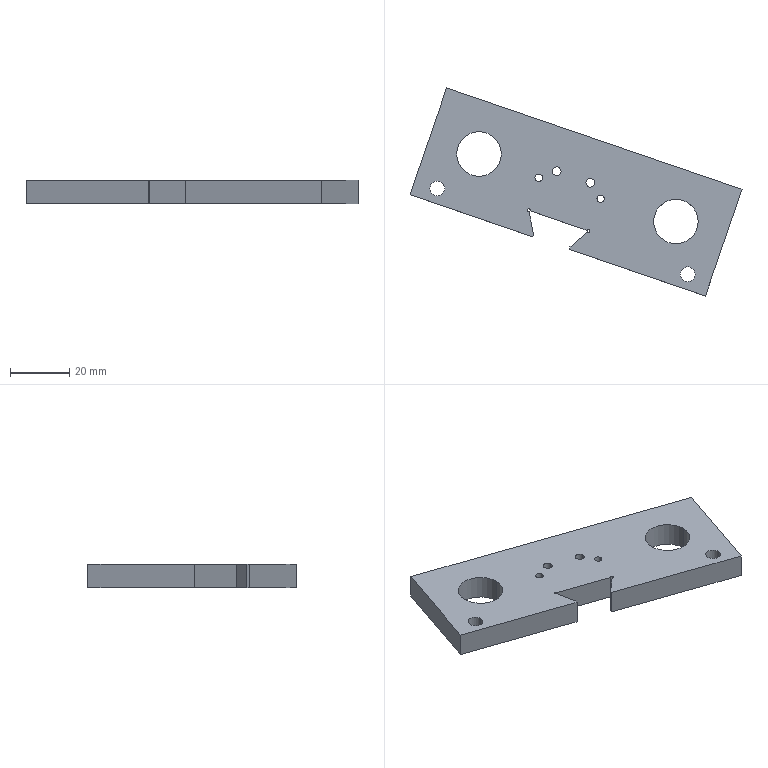Part | SolidWorks | features HoleWzd 3, ICE 3, Cut 1, Extrusion 1 | 1 solid | 33 faces | box 111.649 x 70.016 x 8 mm | volume 27509 mm3 | cylinder 21 | plane 12 | commonest cylinder face diameters 1 x5 2.5 x4 3 x4 5 x4 15 x4
STEP:
#1=CARTESIAN_POINT('',(-174.409,177.441,0.));
#2=VERTEX_POINT('',#1);
#3=CARTESIAN_POINT('',(-175.382,177.604,0.));
#4=VERTEX_POINT('',#3);
#5=CARTESIAN_POINT('',(-174.909,177.441,0.));
#6=DIRECTION('',(0.,0.,1.));
#7=DIRECTION('',(1.,0.,0.));
#8=AXIS2_PLACEMENT_3D('',#5,#6,#7);
#9=CIRCLE('',#8,0.5);
#10=EDGE_CURVE('',#2,#4,#9,.T.);
#11=ORIENTED_EDGE('',*,*,#10,.F.);
#12=CARTESIAN_POINT('',(-174.409,177.441,8.));
#13=VERTEX_POINT('',#12);
#14=CARTESIAN_POINT('',(-174.409,177.441,0.));
#15=DIRECTION('',(0.,0.,1.));
#16=VECTOR('',#15,1000.);
#17=LINE('',#14,#16);
#18=EDGE_CURVE('',#2,#13,#17,.T.);
#19=ORIENTED_EDGE('',*,*,#18,.T.);
#20=CARTESIAN_POINT('',(-175.382,177.604,8.));
#21=VERTEX_POINT('',#20);
#22=CARTESIAN_POINT('',(-174.909,177.441,8.));
#23=DIRECTION('',(0.,0.,1.));
#24=DIRECTION('',(1.,0.,0.));
#25=AXIS2_PLACEMENT_3D('',#22,#23,#24);
#26=CIRCLE('',#25,0.5);
#27=EDGE_CURVE('',#13,#21,#26,.T.);
#28=ORIENTED_EDGE('',*,*,#27,.T.);
#29=CARTESIAN_POINT('',(-175.382,177.604,0.));
#30=DIRECTION('',(0.,0.,1.));
#31=VECTOR('',#30,1000.);
#32=LINE('',#29,#31);
#33=EDGE_CURVE('',#4,#21,#32,.T.);
#34=ORIENTED_EDGE('',*,*,#33,.F.);
#35=EDGE_LOOP('',(#11,#19,#28,#34));
#36=FACE_OUTER_BOUND('',#35,.T.);
#37=CARTESIAN_POINT('',(-174.909,177.441,0.));
#38=DIRECTION('',(0.,0.,1.));
#39=DIRECTION('',(1.,0.,0.));
#40=AXIS2_PLACEMENT_3D('',#37,#38,#39);
#41=CYLINDRICAL_SURFACE('',#40,0.5);
#42=ADVANCED_FACE('',(#36),#41,.F.);
#43=CARTESIAN_POINT('',(-195.497,184.333,0.));
#44=VERTEX_POINT('',#43);
#45=CARTESIAN_POINT('',(-194.901,183.842,0.));
#46=VERTEX_POINT('',#45);
#47=CARTESIAN_POINT('',(-194.997,184.333,0.));
#48=DIRECTION('',(0.,0.,1.));
#49=DIRECTION('',(1.,0.,0.));
#50=AXIS2_PLACEMENT_3D('',#47,#48,#49);
#51=CIRCLE('',#50,0.5);
#52=EDGE_CURVE('',#44,#46,#51,.T.);
#53=ORIENTED_EDGE('',*,*,#52,.F.);
#54=CARTESIAN_POINT('',(-195.497,184.333,8.));
#55=VERTEX_POINT('',#54);
#56=CARTESIAN_POINT('',(-195.497,184.333,0.));
#57=DIRECTION('',(0.,0.,1.));
#58=VECTOR('',#57,1000.);
#59=LINE('',#56,#58);
#60=EDGE_CURVE('',#44,#55,#59,.T.);
#61=ORIENTED_EDGE('',*,*,#60,.T.);
#62=CARTESIAN_POINT('',(-194.901,183.842,8.));
#63=VERTEX_POINT('',#62);
#64=CARTESIAN_POINT('',(-194.997,184.333,8.));
#65=DIRECTION('',(0.,0.,1.));
#66=DIRECTION('',(1.,0.,0.));
#67=AXIS2_PLACEMENT_3D('',#64,#65,#66);
#68=CIRCLE('',#67,0.5);
#69=EDGE_CURVE('',#55,#63,#68,.T.);
#70=ORIENTED_EDGE('',*,*,#69,.T.);
#71=CARTESIAN_POINT('',(-194.901,183.842,0.));
#72=DIRECTION('',(0.,0.,1.));
#73=VECTOR('',#72,1000.);
#74=LINE('',#71,#73);
#75=EDGE_CURVE('',#46,#63,#74,.T.);
#76=ORIENTED_EDGE('',*,*,#75,.F.);
#77=EDGE_LOOP('',(#53,#61,#70,#76));
#78=FACE_OUTER_BOUND('',#77,.T.);
#79=CARTESIAN_POINT('',(-194.997,184.333,0.));
#80=DIRECTION('',(0.,0.,1.));
#81=DIRECTION('',(1.,0.,0.));
#82=AXIS2_PLACEMENT_3D('',#79,#80,#81);
#83=CYLINDRICAL_SURFACE('',#82,0.5);
#84=ADVANCED_FACE('',(#78),#83,.F.);
#85=ORIENTED_EDGE('',*,*,#60,.F.);
#86=CARTESIAN_POINT('',(-194.497,184.333,0.));
#87=VERTEX_POINT('',#86);
#88=CARTESIAN_POINT('',(-194.997,184.333,0.));
#89=DIRECTION('',(0.,0.,1.));
#90=DIRECTION('',(1.,0.,0.));
#91=AXIS2_PLACEMENT_3D('',#88,#89,#90);
#92=CIRCLE('',#91,0.5);
#93=EDGE_CURVE('',#87,#44,#92,.T.);
#94=ORIENTED_EDGE('',*,*,#93,.F.);
#95=CARTESIAN_POINT('',(-194.497,184.333,8.));
#96=VERTEX_POINT('',#95);
#97=CARTESIAN_POINT('',(-194.497,184.333,0.));
#98=DIRECTION('',(0.,0.,1.));
#99=VECTOR('',#98,1000.);
#100=LINE('',#97,#99);
#101=EDGE_CURVE('',#87,#96,#100,.T.);
#102=ORIENTED_EDGE('',*,*,#101,.T.);
#103=CARTESIAN_POINT('',(-194.997,184.333,8.));
#104=DIRECTION('',(0.,0.,1.));
#105=DIRECTION('',(1.,0.,0.));
#106=AXIS2_PLACEMENT_3D('',#103,#104,#105);
#107=CIRCLE('',#106,0.5);
#108=EDGE_CURVE('',#96,#55,#107,.T.);
#109=ORIENTED_EDGE('',*,*,#108,.T.);
#110=EDGE_LOOP('',(#85,#94,#102,#109));
#111=FACE_OUTER_BOUND('',#110,.T.);
#112=CARTESIAN_POINT('',(-194.997,184.333,0.));
#113=DIRECTION('',(0.,0.,1.));
#114=DIRECTION('',(1.,0.,0.));
#115=AXIS2_PLACEMENT_3D('',#112,#113,#114);
#116=CYLINDRICAL_SURFACE('',#115,0.5);
#117=ADVANCED_FACE('',(#111),#116,.F.);
#118=CARTESIAN_POINT('',(-172.756,193.59,8.));
#119=VERTEX_POINT('',#118);
#120=CARTESIAN_POINT('',(-175.756,193.59,8.));
#121=VERTEX_POINT('',#120);
#122=CARTESIAN_POINT('',(-174.256,193.59,8.));
#123=DIRECTION('',(0.,0.,-1.));
#124=DIRECTION('',(-1.,0.,0.));
#125=AXIS2_PLACEMENT_3D('',#122,#123,#124);
#126=CIRCLE('',#125,1.5);
#127=EDGE_CURVE('',#119,#121,#126,.T.);
#128=ORIENTED_EDGE('',*,*,#127,.F.);
#129=CARTESIAN_POINT('',(-172.756,193.59,0.));
#130=VERTEX_POINT('',#129);
#131=CARTESIAN_POINT('',(-172.756,193.59,0.));
#132=DIRECTION('',(0.,0.,-1.));
#133=VECTOR('',#132,1000.);
#134=LINE('',#131,#133);
#135=EDGE_CURVE('',#119,#130,#134,.T.);
#136=ORIENTED_EDGE('',*,*,#135,.T.);
#137=CARTESIAN_POINT('',(-175.756,193.59,0.));
#138=VERTEX_POINT('',#137);
#139=CARTESIAN_POINT('',(-174.256,193.59,0.));
#140=DIRECTION('',(0.,0.,-1.));
#141=DIRECTION('',(-1.,0.,0.));
#142=AXIS2_PLACEMENT_3D('',#139,#140,#141);
#143=CIRCLE('',#142,1.5);
#144=EDGE_CURVE('',#130,#138,#143,.T.);
#145=ORIENTED_EDGE('',*,*,#144,.T.);
#146=CARTESIAN_POINT('',(-175.756,193.59,0.));
#147=DIRECTION('',(0.,0.,-1.));
#148=VECTOR('',#147,1000.);
#149=LINE('',#146,#148);
#150=EDGE_CURVE('',#121,#138,#149,.T.);
#151=ORIENTED_EDGE('',*,*,#150,.F.);
#152=EDGE_LOOP('',(#128,#136,#145,#151));
#153=FACE_OUTER_BOUND('',#152,.T.);
#154=CARTESIAN_POINT('',(-174.256,193.59,0.));
#155=DIRECTION('',(0.,0.,-1.));
#156=DIRECTION('',(-1.,0.,0.));
#157=AXIS2_PLACEMENT_3D('',#154,#155,#156);
#158=CYLINDRICAL_SURFACE('',#157,1.5);
#159=ADVANCED_FACE('',(#153),#158,.F.);
#160=CARTESIAN_POINT('',(-184.111,197.473,8.));
#161=VERTEX_POINT('',#160);
#162=CARTESIAN_POINT('',(-187.111,197.473,8.));
#163=VERTEX_POINT('',#162);
#164=CARTESIAN_POINT('',(-185.611,197.473,8.));
#165=DIRECTION('',(0.,0.,-1.));
#166=DIRECTION('',(-1.,0.,0.));
#167=AXIS2_PLACEMENT_3D('',#164,#165,#166);
#168=CIRCLE('',#167,1.5);
#169=EDGE_CURVE('',#161,#163,#168,.T.);
#170=ORIENTED_EDGE('',*,*,#169,.F.);
#171=CARTESIAN_POINT('',(-184.111,197.473,0.));
#172=VERTEX_POINT('',#171);
#173=CARTESIAN_POINT('',(-184.111,197.473,0.));
#174=DIRECTION('',(0.,0.,-1.));
#175=VECTOR('',#174,1000.);
#176=LINE('',#173,#175);
#177=EDGE_CURVE('',#161,#172,#176,.T.);
#178=ORIENTED_EDGE('',*,*,#177,.T.);
#179=CARTESIAN_POINT('',(-187.111,197.473,0.));
#180=VERTEX_POINT('',#179);
#181=CARTESIAN_POINT('',(-185.611,197.473,0.));
#182=DIRECTION('',(0.,0.,-1.));
#183=DIRECTION('',(-1.,0.,0.));
#184=AXIS2_PLACEMENT_3D('',#181,#182,#183);
#185=CIRCLE('',#184,1.5);
#186=EDGE_CURVE('',#172,#180,#185,.T.);
#187=ORIENTED_EDGE('',*,*,#186,.T.);
#188=CARTESIAN_POINT('',(-187.111,197.473,0.));
#189=DIRECTION('',(0.,0.,-1.));
#190=VECTOR('',#189,1000.);
#191=LINE('',#188,#190);
#192=EDGE_CURVE('',#163,#180,#191,.T.);
#193=ORIENTED_EDGE('',*,*,#192,.F.);
#194=EDGE_LOOP('',(#170,#178,#187,#193));
#195=FACE_OUTER_BOUND('',#194,.T.);
#196=CARTESIAN_POINT('',(-185.611,197.473,0.));
#197=DIRECTION('',(0.,0.,-1.));
#198=DIRECTION('',(-1.,0.,0.));
#199=AXIS2_PLACEMENT_3D('',#196,#197,#198);
#200=CYLINDRICAL_SURFACE('',#199,1.5);
#201=ADVANCED_FACE('',(#195),#200,.F.);
#202=CARTESIAN_POINT('',(-169.569,188.188,8.));
#203=VERTEX_POINT('',#202);
#204=CARTESIAN_POINT('',(-172.069,188.188,8.));
#205=VERTEX_POINT('',#204);
#206=CARTESIAN_POINT('',(-170.819,188.188,8.));
#207=DIRECTION('',(0.,0.,-1.));
#208=DIRECTION('',(-1.,0.,0.));
#209=AXIS2_PLACEMENT_3D('',#206,#207,#208);
#210=CIRCLE('',#209,1.25);
#211=EDGE_CURVE('',#203,#205,#210,.T.);
#212=ORIENTED_EDGE('',*,*,#211,.F.);
#213=CARTESIAN_POINT('',(-169.569,188.188,0.));
#214=VERTEX_POINT('',#213);
#215=CARTESIAN_POINT('',(-169.569,188.188,0.));
#216=DIRECTION('',(0.,0.,-1.));
#217=VECTOR('',#216,1000.);
#218=LINE('',#215,#217);
#219=EDGE_CURVE('',#203,#214,#218,.T.);
#220=ORIENTED_EDGE('',*,*,#219,.T.);
#221=CARTESIAN_POINT('',(-172.069,188.188,0.));
#222=VERTEX_POINT('',#221);
#223=CARTESIAN_POINT('',(-170.819,188.188,0.));
#224=DIRECTION('',(0.,0.,-1.));
#225=DIRECTION('',(-1.,0.,0.));
#226=AXIS2_PLACEMENT_3D('',#223,#224,#225);
#227=CIRCLE('',#226,1.25);
#228=EDGE_CURVE('',#214,#222,#227,.T.);
#229=ORIENTED_EDGE('',*,*,#228,.T.);
#230=CARTESIAN_POINT('',(-172.069,188.188,0.));
#231=DIRECTION('',(0.,0.,-1.));
#232=VECTOR('',#231,1000.);
#233=LINE('',#230,#232);
#234=EDGE_CURVE('',#205,#222,#233,.T.);
#235=ORIENTED_EDGE('',*,*,#234,.F.);
#236=EDGE_LOOP('',(#212,#220,#229,#235));
#237=FACE_OUTER_BOUND('',#236,.T.);
#238=CARTESIAN_POINT('',(-170.819,188.188,0.));
#239=DIRECTION('',(0.,0.,-1.));
#240=DIRECTION('',(-1.,0.,0.));
#241=AXIS2_PLACEMENT_3D('',#238,#239,#240);
#242=CYLINDRICAL_SURFACE('',#241,1.25);
#243=ADVANCED_FACE('',(#237),#242,.F.);
#244=CARTESIAN_POINT('',(-190.386,195.307,8.));
#245=VERTEX_POINT('',#244);
#246=CARTESIAN_POINT('',(-192.886,195.307,8.));
#247=VERTEX_POINT('',#246);
#248=CARTESIAN_POINT('',(-191.636,195.307,8.));
#249=DIRECTION('',(0.,0.,-1.));
#250=DIRECTION('',(-1.,0.,0.));
#251=AXIS2_PLACEMENT_3D('',#248,#249,#250);
#252=CIRCLE('',#251,1.25);
#253=EDGE_CURVE('',#245,#247,#252,.T.);
#254=ORIENTED_EDGE('',*,*,#253,.F.);
#255=CARTESIAN_POINT('',(-190.386,195.307,0.));
#256=VERTEX_POINT('',#255);
#257=CARTESIAN_POINT('',(-190.386,195.307,0.));
#258=DIRECTION('',(0.,0.,-1.));
#259=VECTOR('',#258,1000.);
#260=LINE('',#257,#259);
#261=EDGE_CURVE('',#245,#256,#260,.T.);
#262=ORIENTED_EDGE('',*,*,#261,.T.);
#263=CARTESIAN_POINT('',(-192.886,195.307,0.));
#264=VERTEX_POINT('',#263);
#265=CARTESIAN_POINT('',(-191.636,195.307,0.));
#266=DIRECTION('',(0.,0.,-1.));
#267=DIRECTION('',(-1.,0.,0.));
#268=AXIS2_PLACEMENT_3D('',#265,#266,#267);
#269=CIRCLE('',#268,1.25);
#270=EDGE_CURVE('',#256,#264,#269,.T.);
#271=ORIENTED_EDGE('',*,*,#270,.T.);
#272=CARTESIAN_POINT('',(-192.886,195.307,0.));
#273=DIRECTION('',(0.,0.,-1.));
#274=VECTOR('',#273,1000.);
#275=LINE('',#272,#274);
#276=EDGE_CURVE('',#247,#264,#275,.T.);
#277=ORIENTED_EDGE('',*,*,#276,.F.);
#278=EDGE_LOOP('',(#254,#262,#271,#277));
#279=FACE_OUTER_BOUND('',#278,.T.);
#280=CARTESIAN_POINT('',(-191.636,195.307,0.));
#281=DIRECTION('',(0.,0.,-1.));
#282=DIRECTION('',(-1.,0.,0.));
#283=AXIS2_PLACEMENT_3D('',#280,#281,#282);
#284=CYLINDRICAL_SURFACE('',#283,1.25);
#285=ADVANCED_FACE('',(#279),#284,.F.);
#286=CARTESIAN_POINT('',(-144.049,162.825,0.));
#287=VERTEX_POINT('',#286);
#288=CARTESIAN_POINT('',(-139.049,162.825,0.));
#289=VERTEX_POINT('',#288);
#290=CARTESIAN_POINT('',(-141.549,162.825,0.));
#291=DIRECTION('',(0.,0.,1.));
#292=DIRECTION('',(1.,0.,0.));
#293=AXIS2_PLACEMENT_3D('',#290,#291,#292);
#294=CIRCLE('',#293,2.5);
#295=EDGE_CURVE('',#287,#289,#294,.T.);
#296=ORIENTED_EDGE('',*,*,#295,.F.);
#297=CARTESIAN_POINT('',(-144.049,162.825,8.));
#298=VERTEX_POINT('',#297);
#299=CARTESIAN_POINT('',(-144.049,162.825,8.));
#300=DIRECTION('',(0.,0.,1.));
#301=VECTOR('',#300,1000.);
#302=LINE('',#299,#301);
#303=EDGE_CURVE('',#287,#298,#302,.T.);
#304=ORIENTED_EDGE('',*,*,#303,.T.);
#305=CARTESIAN_POINT('',(-139.049,162.825,8.));
#306=VERTEX_POINT('',#305);
#307=CARTESIAN_POINT('',(-141.549,162.825,8.));
#308=DIRECTION('',(0.,0.,1.));
#309=DIRECTION('',(1.,0.,0.));
#310=AXIS2_PLACEMENT_3D('',#307,#308,#309);
#311=CIRCLE('',#310,2.5);
#312=EDGE_CURVE('',#298,#306,#311,.T.);
#313=ORIENTED_EDGE('',*,*,#312,.T.);
#314=CARTESIAN_POINT('',(-139.049,162.825,8.));
#315=DIRECTION('',(0.,0.,1.));
#316=VECTOR('',#315,1000.);
#317=LINE('',#314,#316);
#318=EDGE_CURVE('',#289,#306,#317,.T.);
#319=ORIENTED_EDGE('',*,*,#318,.F.);
#320=EDGE_LOOP('',(#296,#304,#313,#319));
#321=FACE_OUTER_BOUND('',#320,.T.);
#322=CARTESIAN_POINT('',(-141.549,162.825,8.));
#323=DIRECTION('',(0.,0.,1.));
#324=DIRECTION('',(1.,0.,0.));
#325=AXIS2_PLACEMENT_3D('',#322,#323,#324);
#326=CYLINDRICAL_SURFACE('',#325,2.5);
#327=ADVANCED_FACE('',(#321),#326,.F.);
#328=CARTESIAN_POINT('',(-228.232,191.705,0.));
#329=VERTEX_POINT('',#328);
#330=CARTESIAN_POINT('',(-223.232,191.705,0.));
#331=VERTEX_POINT('',#330);
#332=CARTESIAN_POINT('',(-225.732,191.705,0.));
#333=DIRECTION('',(0.,0.,1.));
#334=DIRECTION('',(1.,0.,0.));
#335=AXIS2_PLACEMENT_3D('',#332,#333,#334);
#336=CIRCLE('',#335,2.5);
#337=EDGE_CURVE('',#329,#331,#336,.T.);
#338=ORIENTED_EDGE('',*,*,#337,.F.);
#339=CARTESIAN_POINT('',(-228.232,191.705,8.));
#340=VERTEX_POINT('',#339);
#341=CARTESIAN_POINT('',(-228.232,191.705,8.));
#342=DIRECTION('',(0.,0.,1.));
#343=VECTOR('',#342,1000.);
#344=LINE('',#341,#343);
#345=EDGE_CURVE('',#329,#340,#344,.T.);
#346=ORIENTED_EDGE('',*,*,#345,.T.);
#347=CARTESIAN_POINT('',(-223.232,191.705,8.));
#348=VERTEX_POINT('',#347);
#349=CARTESIAN_POINT('',(-225.732,191.705,8.));
#350=DIRECTION('',(0.,0.,1.));
#351=DIRECTION('',(1.,0.,0.));
#352=AXIS2_PLACEMENT_3D('',#349,#350,#351);
#353=CIRCLE('',#352,2.5);
#354=EDGE_CURVE('',#340,#348,#353,.T.);
#355=ORIENTED_EDGE('',*,*,#354,.T.);
#356=CARTESIAN_POINT('',(-223.232,191.705,8.));
#357=DIRECTION('',(0.,0.,1.));
#358=VECTOR('',#357,1000.);
#359=LINE('',#356,#358);
#360=EDGE_CURVE('',#331,#348,#359,.T.);
#361=ORIENTED_EDGE('',*,*,#360,.F.);
#362=EDGE_LOOP('',(#338,#346,#355,#361));
#363=FACE_OUTER_BOUND('',#362,.T.);
#364=CARTESIAN_POINT('',(-225.732,191.705,8.));
#365=DIRECTION('',(0.,0.,1.));
#366=DIRECTION('',(1.,0.,0.));
#367=AXIS2_PLACEMENT_3D('',#364,#365,#366);
#368=CYLINDRICAL_SURFACE('',#367,2.5);
#369=ADVANCED_FACE('',(#363),#368,.F.);
#370=CARTESIAN_POINT('',(-138.005,180.569,8.));
#371=VERTEX_POINT('',#370);
#372=CARTESIAN_POINT('',(-153.005,180.569,8.));
#373=VERTEX_POINT('',#372);
#374=CARTESIAN_POINT('',(-145.505,180.569,8.));
#375=DIRECTION('',(0.,0.,-1.));
#376=DIRECTION('',(0.,1.,0.));
#377=AXIS2_PLACEMENT_3D('',#374,#375,#376);
#378=CIRCLE('',#377,7.5);
#379=EDGE_CURVE('',#371,#373,#378,.T.);
#380=ORIENTED_EDGE('',*,*,#379,.F.);
#381=CARTESIAN_POINT('',(-138.005,180.569,0.));
#382=VERTEX_POINT('',#381);
#383=CARTESIAN_POINT('',(-138.005,180.569,137.468));
#384=DIRECTION('',(0.,0.,-1.));
#385=VECTOR('',#384,1000.);
#386=LINE('',#383,#385);
#387=EDGE_CURVE('',#371,#382,#386,.T.);
#388=ORIENTED_EDGE('',*,*,#387,.T.);
#389=CARTESIAN_POINT('',(-153.005,180.569,0.));
#390=VERTEX_POINT('',#389);
#391=CARTESIAN_POINT('',(-145.505,180.569,0.));
#392=DIRECTION('',(0.,0.,1.));
#393=DIRECTION('',(1.,0.,0.));
#394=AXIS2_PLACEMENT_3D('',#391,#392,#393);
#395=CIRCLE('',#394,7.5);
#396=EDGE_CURVE('',#390,#382,#395,.T.);
#397=ORIENTED_EDGE('',*,*,#396,.F.);
#398=CARTESIAN_POINT('',(-153.005,180.569,137.468));
#399=DIRECTION('',(0.,0.,-1.));
#400=VECTOR('',#399,1000.);
#401=LINE('',#398,#400);
#402=EDGE_CURVE('',#373,#390,#401,.T.);
#403=ORIENTED_EDGE('',*,*,#402,.F.);
#404=EDGE_LOOP('',(#380,#388,#397,#403));
#405=FACE_OUTER_BOUND('',#404,.T.);
#406=CARTESIAN_POINT('',(-145.505,180.569,137.468));
#407=DIRECTION('',(0.,0.,-1.));
#408=DIRECTION('',(-1.,0.,0.));
#409=AXIS2_PLACEMENT_3D('',#406,#407,#408);
#410=CYLINDRICAL_SURFACE('',#409,7.5);
#411=ADVANCED_FACE('',(#405),#410,.F.);
#412=CARTESIAN_POINT('',(-204.217,203.284,8.));
#413=VERTEX_POINT('',#412);
#414=CARTESIAN_POINT('',(-219.217,203.284,8.));
#415=VERTEX_POINT('',#414);
#416=CARTESIAN_POINT('',(-211.717,203.284,8.));
#417=DIRECTION('',(0.,0.,-1.));
#418=DIRECTION('',(0.,1.,0.));
#419=AXIS2_PLACEMENT_3D('',#416,#417,#418);
#420=CIRCLE('',#419,7.5);
#421=EDGE_CURVE('',#413,#415,#420,.T.);
#422=ORIENTED_EDGE('',*,*,#421,.F.);
#423=CARTESIAN_POINT('',(-204.217,203.284,0.));
#424=VERTEX_POINT('',#423);
#425=CARTESIAN_POINT('',(-204.217,203.284,137.468));
#426=DIRECTION('',(0.,0.,-1.));
#427=VECTOR('',#426,1000.);
#428=LINE('',#425,#427);
#429=EDGE_CURVE('',#413,#424,#428,.T.);
#430=ORIENTED_EDGE('',*,*,#429,.T.);
#431=CARTESIAN_POINT('',(-219.217,203.284,0.));
#432=VERTEX_POINT('',#431);
#433=CARTESIAN_POINT('',(-211.717,203.284,0.));
#434=DIRECTION('',(0.,0.,1.));
#435=DIRECTION('',(1.,0.,0.));
#436=AXIS2_PLACEMENT_3D('',#433,#434,#435);
#437=CIRCLE('',#436,7.5);
#438=EDGE_CURVE('',#432,#424,#437,.T.);
#439=ORIENTED_EDGE('',*,*,#438,.F.);
#440=CARTESIAN_POINT('',(-219.217,203.284,137.468));
#441=DIRECTION('',(0.,0.,-1.));
#442=VECTOR('',#441,1000.);
#443=LINE('',#440,#442);
#444=EDGE_CURVE('',#415,#432,#443,.T.);
#445=ORIENTED_EDGE('',*,*,#444,.F.);
#446=EDGE_LOOP('',(#422,#430,#439,#445));
#447=FACE_OUTER_BOUND('',#446,.T.);
#448=CARTESIAN_POINT('',(-211.717,203.284,137.468));
#449=DIRECTION('',(0.,0.,-1.));
#450=DIRECTION('',(-1.,0.,0.));
#451=AXIS2_PLACEMENT_3D('',#448,#449,#450);
#452=CYLINDRICAL_SURFACE('',#451,7.5);
#453=ADVANCED_FACE('',(#447),#452,.F.);
#454=CARTESIAN_POINT('',(-181.401,171.211,0.));
#455=VERTEX_POINT('',#454);
#456=CARTESIAN_POINT('',(-181.401,171.211,8.));
#457=VERTEX_POINT('',#456);
#458=CARTESIAN_POINT('',(-181.401,171.211,-2.));
#459=DIRECTION('',(0.,0.,1.));
#460=VECTOR('',#459,1000.);
#461=LINE('',#458,#460);
#462=EDGE_CURVE('',#455,#457,#461,.T.);
#463=ORIENTED_EDGE('',*,*,#462,.F.);
#464=CARTESIAN_POINT('',(-135.604,155.5,0.));
#465=VERTEX_POINT('',#464);
#466=CARTESIAN_POINT('',(-234.922,189.572,0.));
#467=DIRECTION('',(0.9459,-0.3245,0.));
#468=VECTOR('',#467,1000.);
#469=LINE('',#466,#468);
#470=EDGE_CURVE('',#455,#465,#469,.T.);
#471=ORIENTED_EDGE('',*,*,#470,.T.);
#472=CARTESIAN_POINT('',(-135.604,155.5,8.));
#473=VERTEX_POINT('',#472);
#474=CARTESIAN_POINT('',(-135.604,155.5,0.));
#475=DIRECTION('',(0.,0.,1.));
#476=VECTOR('',#475,1000.);
#477=LINE('',#474,#476);
#478=EDGE_CURVE('',#465,#473,#477,.T.);
#479=ORIENTED_EDGE('',*,*,#478,.T.);
#480=CARTESIAN_POINT('',(-135.604,155.5,8.));
#481=DIRECTION('',(-0.9459,0.3245,0.));
#482=VECTOR('',#481,1000.);
#483=LINE('',#480,#482);
#484=EDGE_CURVE('',#473,#457,#483,.T.);
#485=ORIENTED_EDGE('',*,*,#484,.T.);
#486=EDGE_LOOP('',(#463,#471,#479,#485));
#487=FACE_OUTER_BOUND('',#486,.T.);
#488=CARTESIAN_POINT('',(33.45,97.503,0.));
#489=DIRECTION('',(-0.3245,-0.9459,0.));
#490=DIRECTION('',(0.9459,-0.3245,0.));
#491=AXIS2_PLACEMENT_3D('',#488,#489,#490);
#492=PLANE('',#491);
#493=ADVANCED_FACE('',(#487),#492,.T.);
#494=CARTESIAN_POINT('',(-174.256,193.59,0.));
#495=DIRECTION('',(0.,0.,-1.));
#496=DIRECTION('',(-1.,0.,0.));
#497=AXIS2_PLACEMENT_3D('',#494,#495,#496);
#498=CIRCLE('',#497,1.5);
#499=EDGE_CURVE('',#138,#130,#498,.T.);
#500=ORIENTED_EDGE('',*,*,#499,.F.);
#501=ORIENTED_EDGE('',*,*,#144,.F.);
#502=EDGE_LOOP('',(#500,#501));
#503=FACE_BOUND('',#502,.T.);
#504=CARTESIAN_POINT('',(-185.611,197.473,0.));
#505=DIRECTION('',(0.,0.,-1.));
#506=DIRECTION('',(-1.,0.,0.));
#507=AXIS2_PLACEMENT_3D('',#504,#505,#506);
#508=CIRCLE('',#507,1.5);
#509=EDGE_CURVE('',#180,#172,#508,.T.);
#510=ORIENTED_EDGE('',*,*,#509,.F.);
#511=ORIENTED_EDGE('',*,*,#186,.F.);
#512=EDGE_LOOP('',(#510,#511));
#513=FACE_BOUND('',#512,.T.);
#514=CARTESIAN_POINT('',(-170.819,188.188,0.));
#515=DIRECTION('',(0.,0.,-1.));
#516=DIRECTION('',(-1.,0.,0.));
#517=AXIS2_PLACEMENT_3D('',#514,#515,#516);
#518=CIRCLE('',#517,1.25);
#519=EDGE_CURVE('',#222,#214,#518,.T.);
#520=ORIENTED_EDGE('',*,*,#519,.F.);
#521=ORIENTED_EDGE('',*,*,#228,.F.);
#522=EDGE_LOOP('',(#520,#521));
#523=FACE_BOUND('',#522,.T.);
#524=CARTESIAN_POINT('',(-191.636,195.307,0.));
#525=DIRECTION('',(0.,0.,-1.));
#526=DIRECTION('',(-1.,0.,0.));
#527=AXIS2_PLACEMENT_3D('',#524,#525,#526);
#528=CIRCLE('',#527,1.25);
#529=EDGE_CURVE('',#264,#256,#528,.T.);
#530=ORIENTED_EDGE('',*,*,#529,.F.);
#531=ORIENTED_EDGE('',*,*,#270,.F.);
#532=EDGE_LOOP('',(#530,#531));
#533=FACE_BOUND('',#532,.T.);
#534=CARTESIAN_POINT('',(-141.549,162.825,0.));
#535=DIRECTION('',(0.,0.,1.));
#536=DIRECTION('',(1.,0.,0.));
#537=AXIS2_PLACEMENT_3D('',#534,#535,#536);
#538=CIRCLE('',#537,2.5);
#539=EDGE_CURVE('',#289,#287,#538,.T.);
#540=ORIENTED_EDGE('',*,*,#539,.T.);
#541=ORIENTED_EDGE('',*,*,#295,.T.);
#542=EDGE_LOOP('',(#540,#541));
#543=FACE_BOUND('',#542,.T.);
#544=CARTESIAN_POINT('',(-225.732,191.705,0.));
#545=DIRECTION('',(0.,0.,1.));
#546=DIRECTION('',(1.,0.,0.));
#547=AXIS2_PLACEMENT_3D('',#544,#545,#546);
#548=CIRCLE('',#547,2.5);
#549=EDGE_CURVE('',#331,#329,#548,.T.);
#550=ORIENTED_EDGE('',*,*,#549,.T.);
#551=ORIENTED_EDGE('',*,*,#337,.T.);
#552=EDGE_LOOP('',(#550,#551));
#553=FACE_BOUND('',#552,.T.);
#554=CARTESIAN_POINT('',(-181.12,172.03,0.));
#555=VERTEX_POINT('',#554);
#556=CARTESIAN_POINT('',(-175.286,177.113,0.));
#557=VERTEX_POINT('',#556);
#558=CARTESIAN_POINT('',(-181.874,171.373,0.));
#559=DIRECTION('',(0.754,0.6569,0.));
#560=VECTOR('',#559,1000.);
#561=LINE('',#558,#560);
#562=EDGE_CURVE('',#555,#557,#561,.T.);
#563=ORIENTED_EDGE('',*,*,#562,.T.);
#564=CARTESIAN_POINT('',(-174.909,177.441,0.));
#565=DIRECTION('',(0.,0.,1.));
#566=DIRECTION('',(1.,0.,0.));
#567=AXIS2_PLACEMENT_3D('',#564,#565,#566);
#568=CIRCLE('',#567,0.5);
#569=EDGE_CURVE('',#557,#2,#568,.T.);
#570=ORIENTED_EDGE('',*,*,#569,.T.);
#571=ORIENTED_EDGE('',*,*,#10,.T.);
#572=CARTESIAN_POINT('',(-194.524,184.171,0.));
#573=VERTEX_POINT('',#572);
#574=CARTESIAN_POINT('',(-174.909,177.441,0.));
#575=DIRECTION('',(-0.9459,0.3245,0.));
#576=VECTOR('',#575,1000.);
#577=LINE('',#574,#576);
#578=EDGE_CURVE('',#4,#573,#577,.T.);
#579=ORIENTED_EDGE('',*,*,#578,.T.);
#580=CARTESIAN_POINT('',(-194.997,184.333,0.));
#581=DIRECTION('',(0.,0.,1.));
#582=DIRECTION('',(1.,0.,0.));
#583=AXIS2_PLACEMENT_3D('',#580,#581,#582);
#584=CIRCLE('',#583,0.5);
#585=EDGE_CURVE('',#573,#87,#584,.T.);
#586=ORIENTED_EDGE('',*,*,#585,.T.);
#587=ORIENTED_EDGE('',*,*,#93,.T.);
#588=ORIENTED_EDGE('',*,*,#52,.T.);
#589=CARTESIAN_POINT('',(-193.416,176.249,0.));
#590=VERTEX_POINT('',#589);
#591=CARTESIAN_POINT('',(-193.224,175.267,0.));
#592=DIRECTION('',(0.1919,-0.9814,0.));
#593=VECTOR('',#592,1000.);
#594=LINE('',#591,#593);
#595=EDGE_CURVE('',#46,#590,#594,.T.);
#596=ORIENTED_EDGE('',*,*,#595,.T.);
#597=CARTESIAN_POINT('',(-193.697,175.429,0.));
#598=VERTEX_POINT('',#597);
#599=CARTESIAN_POINT('',(-227.147,77.926,0.));
#600=DIRECTION('',(-0.3245,-0.9459,0.));
#601=VECTOR('',#600,1000.);
#602=LINE('',#599,#601);
#603=EDGE_CURVE('',#590,#598,#602,.T.);
#604=ORIENTED_EDGE('',*,*,#603,.T.);
#605=CARTESIAN_POINT('',(-234.922,189.572,0.));
#606=VERTEX_POINT('',#605);
#607=CARTESIAN_POINT('',(-234.922,189.572,0.));
#608=DIRECTION('',(0.9459,-0.3245,0.));
#609=VECTOR('',#608,1000.);
#610=LINE('',#607,#609);
#611=EDGE_CURVE('',#606,#598,#610,.T.);
#612=ORIENTED_EDGE('',*,*,#611,.F.);
#613=CARTESIAN_POINT('',(-222.591,225.516,0.));
#614=VERTEX_POINT('',#613);
#615=CARTESIAN_POINT('',(-222.591,225.516,0.));
#616=DIRECTION('',(-0.3245,-0.9459,0.));
#617=VECTOR('',#616,1000.);
#618=LINE('',#615,#617);
#619=EDGE_CURVE('',#614,#606,#618,.T.);
#620=ORIENTED_EDGE('',*,*,#619,.F.);
#621=CARTESIAN_POINT('',(-123.273,191.443,0.));
#622=VERTEX_POINT('',#621);
#623=CARTESIAN_POINT('',(-123.273,191.443,0.));
#624=DIRECTION('',(-0.9459,0.3245,0.));
#625=VECTOR('',#624,1000.);
#626=LINE('',#623,#625);
#627=EDGE_CURVE('',#622,#614,#626,.T.);
#628=ORIENTED_EDGE('',*,*,#627,.F.);
#629=CARTESIAN_POINT('',(-123.273,191.443,0.));
#630=DIRECTION('',(0.3245,0.9459,0.));
#631=VECTOR('',#630,1000.);
#632=LINE('',#629,#631);
#633=EDGE_CURVE('',#465,#622,#632,.T.);
#634=ORIENTED_EDGE('',*,*,#633,.F.);
#635=ORIENTED_EDGE('',*,*,#470,.F.);
#636=CARTESIAN_POINT('',(-214.851,73.708,0.));
#637=DIRECTION('',(0.3245,0.9459,0.));
#638=VECTOR('',#637,1000.);
#639=LINE('',#636,#638);
#640=EDGE_CURVE('',#455,#555,#639,.T.);
#641=ORIENTED_EDGE('',*,*,#640,.T.);
#642=EDGE_LOOP('',(#563,#570,#571,#579,#586,#587,#588,#596,#604,#612,#620,#628,#634,#635,#641));
#643=FACE_OUTER_BOUND('',#642,.T.);
#644=ORIENTED_EDGE('',*,*,#438,.T.);
#645=CARTESIAN_POINT('',(-211.717,203.284,0.));
#646=DIRECTION('',(0.,0.,1.));
#647=DIRECTION('',(1.,0.,0.));
#648=AXIS2_PLACEMENT_3D('',#645,#646,#647);
#649=CIRCLE('',#648,7.5);
#650=EDGE_CURVE('',#424,#432,#649,.T.);
#651=ORIENTED_EDGE('',*,*,#650,.T.);
#652=EDGE_LOOP('',(#644,#651));
#653=FACE_BOUND('',#652,.T.);
#654=ORIENTED_EDGE('',*,*,#396,.T.);
#655=CARTESIAN_POINT('',(-145.505,180.569,0.));
#656=DIRECTION('',(0.,0.,1.));
#657=DIRECTION('',(1.,0.,0.));
#658=AXIS2_PLACEMENT_3D('',#655,#656,#657);
#659=CIRCLE('',#658,7.5);
#660=EDGE_CURVE('',#382,#390,#659,.T.);
#661=ORIENTED_EDGE('',*,*,#660,.T.);
#662=EDGE_LOOP('',(#654,#661));
#663=FACE_BOUND('',#662,.T.);
#664=CARTESIAN_POINT('',(0.,0.,0.));
#665=DIRECTION('',(0.,0.,1.));
#666=DIRECTION('',(1.,0.,0.));
#667=AXIS2_PLACEMENT_3D('',#664,#665,#666);
#668=PLANE('',#667);
#669=ADVANCED_FACE('',(#503,#513,#523,#533,#543,#553,#643,#653,#663),#668,.F.);
#670=CARTESIAN_POINT('',(-123.273,191.443,8.));
#671=VERTEX_POINT('',#670);
#672=CARTESIAN_POINT('',(-123.273,191.443,137.468));
#673=DIRECTION('',(0.,0.,-1.));
#674=VECTOR('',#673,1000.);
#675=LINE('',#672,#674);
#676=EDGE_CURVE('',#671,#622,#675,.T.);
#677=ORIENTED_EDGE('',*,*,#676,.F.);
#678=CARTESIAN_POINT('',(-123.273,191.443,8.));
#679=DIRECTION('',(-0.3245,-0.9459,0.));
#680=VECTOR('',#679,1000.);
#681=LINE('',#678,#680);
#682=EDGE_CURVE('',#671,#473,#681,.T.);
#683=ORIENTED_EDGE('',*,*,#682,.T.);
#684=ORIENTED_EDGE('',*,*,#478,.F.);
#685=ORIENTED_EDGE('',*,*,#633,.T.);
#686=EDGE_LOOP('',(#677,#683,#684,#685));
#687=FACE_OUTER_BOUND('',#686,.T.);
#688=CARTESIAN_POINT('',(-123.273,191.443,137.468));
#689=DIRECTION('',(-0.9459,0.3245,0.));
#690=DIRECTION('',(-0.3245,-0.9459,0.));
#691=AXIS2_PLACEMENT_3D('',#688,#689,#690);
#692=PLANE('',#691);
#693=ADVANCED_FACE('',(#687),#692,.F.);
#694=CARTESIAN_POINT('',(-222.591,225.516,8.));
#695=VERTEX_POINT('',#694);
#696=CARTESIAN_POINT('',(-222.591,225.516,137.468));
#697=DIRECTION('',(0.,0.,-1.));
#698=VECTOR('',#697,1000.);
#699=LINE('',#696,#698);
#700=EDGE_CURVE('',#695,#614,#699,.T.);
#701=ORIENTED_EDGE('',*,*,#700,.F.);
#702=CARTESIAN_POINT('',(-123.273,191.443,8.));
#703=DIRECTION('',(0.9459,-0.3245,0.));
#704=VECTOR('',#703,1000.);
#705=LINE('',#702,#704);
#706=EDGE_CURVE('',#695,#671,#705,.T.);
#707=ORIENTED_EDGE('',*,*,#706,.T.);
#708=ORIENTED_EDGE('',*,*,#676,.T.);
#709=ORIENTED_EDGE('',*,*,#627,.T.);
#710=EDGE_LOOP('',(#701,#707,#708,#709));
#711=FACE_OUTER_BOUND('',#710,.T.);
#712=CARTESIAN_POINT('',(-123.273,191.443,137.468));
#713=DIRECTION('',(-0.3245,-0.9459,0.));
#714=DIRECTION('',(0.9459,-0.3245,0.));
#715=AXIS2_PLACEMENT_3D('',#712,#713,#714);
#716=PLANE('',#715);
#717=ADVANCED_FACE('',(#711),#716,.F.);
#718=ORIENTED_EDGE('',*,*,#619,.T.);
#719=CARTESIAN_POINT('',(-234.922,189.572,8.));
#720=VERTEX_POINT('',#719);
#721=CARTESIAN_POINT('',(-234.922,189.572,8.));
#722=DIRECTION('',(0.,0.,-1.));
#723=VECTOR('',#722,1000.);
#724=LINE('',#721,#723);
#725=EDGE_CURVE('',#720,#606,#724,.T.);
#726=ORIENTED_EDGE('',*,*,#725,.F.);
#727=CARTESIAN_POINT('',(-222.591,225.516,8.));
#728=DIRECTION('',(0.3245,0.9459,0.));
#729=VECTOR('',#728,1000.);
#730=LINE('',#727,#729);
#731=EDGE_CURVE('',#720,#695,#730,.T.);
#732=ORIENTED_EDGE('',*,*,#731,.T.);
#733=ORIENTED_EDGE('',*,*,#700,.T.);
#734=EDGE_LOOP('',(#718,#726,#732,#733));
#735=FACE_OUTER_BOUND('',#734,.T.);
#736=CARTESIAN_POINT('',(-222.591,225.516,137.468));
#737=DIRECTION('',(0.9459,-0.3245,0.));
#738=DIRECTION('',(0.3245,0.9459,0.));
#739=AXIS2_PLACEMENT_3D('',#736,#737,#738);
#740=PLANE('',#739);
#741=ADVANCED_FACE('',(#735),#740,.F.);
#742=ORIENTED_EDGE('',*,*,#429,.F.);
#743=CARTESIAN_POINT('',(-211.717,203.284,8.));
#744=DIRECTION('',(0.,0.,-1.));
#745=DIRECTION('',(0.,1.,0.));
#746=AXIS2_PLACEMENT_3D('',#743,#744,#745);
#747=CIRCLE('',#746,7.5);
#748=EDGE_CURVE('',#415,#413,#747,.T.);
#749=ORIENTED_EDGE('',*,*,#748,.F.);
#750=ORIENTED_EDGE('',*,*,#444,.T.);
#751=ORIENTED_EDGE('',*,*,#650,.F.);
#752=EDGE_LOOP('',(#742,#749,#750,#751));
#753=FACE_OUTER_BOUND('',#752,.T.);
#754=CARTESIAN_POINT('',(-211.717,203.284,137.468));
#755=DIRECTION('',(0.,0.,-1.));
#756=DIRECTION('',(-1.,0.,0.));
#757=AXIS2_PLACEMENT_3D('',#754,#755,#756);
#758=CYLINDRICAL_SURFACE('',#757,7.5);
#759=ADVANCED_FACE('',(#753),#758,.F.);
#760=ORIENTED_EDGE('',*,*,#387,.F.);
#761=CARTESIAN_POINT('',(-145.505,180.569,8.));
#762=DIRECTION('',(0.,0.,-1.));
#763=DIRECTION('',(0.,1.,0.));
#764=AXIS2_PLACEMENT_3D('',#761,#762,#763);
#765=CIRCLE('',#764,7.5);
#766=EDGE_CURVE('',#373,#371,#765,.T.);
#767=ORIENTED_EDGE('',*,*,#766,.F.);
#768=ORIENTED_EDGE('',*,*,#402,.T.);
#769=ORIENTED_EDGE('',*,*,#660,.F.);
#770=EDGE_LOOP('',(#760,#767,#768,#769));
#771=FACE_OUTER_BOUND('',#770,.T.);
#772=CARTESIAN_POINT('',(-145.505,180.569,137.468));
#773=DIRECTION('',(0.,0.,-1.));
#774=DIRECTION('',(-1.,0.,0.));
#775=AXIS2_PLACEMENT_3D('',#772,#773,#774);
#776=CYLINDRICAL_SURFACE('',#775,7.5);
#777=ADVANCED_FACE('',(#771),#776,.F.);
#778=CARTESIAN_POINT('',(-174.256,193.59,8.));
#779=DIRECTION('',(0.,0.,-1.));
#780=DIRECTION('',(-1.,0.,0.));
#781=AXIS2_PLACEMENT_3D('',#778,#779,#780);
#782=CIRCLE('',#781,1.5);
#783=EDGE_CURVE('',#121,#119,#782,.T.);
#784=ORIENTED_EDGE('',*,*,#783,.T.);
#785=ORIENTED_EDGE('',*,*,#127,.T.);
#786=EDGE_LOOP('',(#784,#785));
#787=FACE_BOUND('',#786,.T.);
#788=CARTESIAN_POINT('',(-185.611,197.473,8.));
#789=DIRECTION('',(0.,0.,-1.));
#790=DIRECTION('',(-1.,0.,0.));
#791=AXIS2_PLACEMENT_3D('',#788,#789,#790);
#792=CIRCLE('',#791,1.5);
#793=EDGE_CURVE('',#163,#161,#792,.T.);
#794=ORIENTED_EDGE('',*,*,#793,.T.);
#795=ORIENTED_EDGE('',*,*,#169,.T.);
#796=EDGE_LOOP('',(#794,#795));
#797=FACE_BOUND('',#796,.T.);
#798=CARTESIAN_POINT('',(-170.819,188.188,8.));
#799=DIRECTION('',(0.,0.,-1.));
#800=DIRECTION('',(-1.,0.,0.));
#801=AXIS2_PLACEMENT_3D('',#798,#799,#800);
#802=CIRCLE('',#801,1.25);
#803=EDGE_CURVE('',#205,#203,#802,.T.);
#804=ORIENTED_EDGE('',*,*,#803,.T.);
#805=ORIENTED_EDGE('',*,*,#211,.T.);
#806=EDGE_LOOP('',(#804,#805));
#807=FACE_BOUND('',#806,.T.);
#808=CARTESIAN_POINT('',(-191.636,195.307,8.));
#809=DIRECTION('',(0.,0.,-1.));
#810=DIRECTION('',(-1.,0.,0.));
#811=AXIS2_PLACEMENT_3D('',#808,#809,#810);
#812=CIRCLE('',#811,1.25);
#813=EDGE_CURVE('',#247,#245,#812,.T.);
#814=ORIENTED_EDGE('',*,*,#813,.T.);
#815=ORIENTED_EDGE('',*,*,#253,.T.);
#816=EDGE_LOOP('',(#814,#815));
#817=FACE_BOUND('',#816,.T.);
#818=CARTESIAN_POINT('',(-141.549,162.825,8.));
#819=DIRECTION('',(0.,0.,1.));
#820=DIRECTION('',(1.,0.,0.));
#821=AXIS2_PLACEMENT_3D('',#818,#819,#820);
#822=CIRCLE('',#821,2.5);
#823=EDGE_CURVE('',#306,#298,#822,.T.);
#824=ORIENTED_EDGE('',*,*,#823,.F.);
#825=ORIENTED_EDGE('',*,*,#312,.F.);
#826=EDGE_LOOP('',(#824,#825));
#827=FACE_BOUND('',#826,.T.);
#828=CARTESIAN_POINT('',(-225.732,191.705,8.));
#829=DIRECTION('',(0.,0.,1.));
#830=DIRECTION('',(1.,0.,0.));
#831=AXIS2_PLACEMENT_3D('',#828,#829,#830);
#832=CIRCLE('',#831,2.5);
#833=EDGE_CURVE('',#348,#340,#832,.T.);
#834=ORIENTED_EDGE('',*,*,#833,.F.);
#835=ORIENTED_EDGE('',*,*,#354,.F.);
#836=EDGE_LOOP('',(#834,#835));
#837=FACE_BOUND('',#836,.T.);
#838=ORIENTED_EDGE('',*,*,#766,.T.);
#839=ORIENTED_EDGE('',*,*,#379,.T.);
#840=EDGE_LOOP('',(#838,#839));
#841=FACE_BOUND('',#840,.T.);
#842=ORIENTED_EDGE('',*,*,#748,.T.);
#843=ORIENTED_EDGE('',*,*,#421,.T.);
#844=EDGE_LOOP('',(#842,#843));
#845=FACE_BOUND('',#844,.T.);
#846=CARTESIAN_POINT('',(-194.524,184.171,8.));
#847=VERTEX_POINT('',#846);
#848=CARTESIAN_POINT('',(-174.909,177.441,8.));
#849=DIRECTION('',(-0.9459,0.3245,0.));
#850=VECTOR('',#849,1000.);
#851=LINE('',#848,#850);
#852=EDGE_CURVE('',#21,#847,#851,.T.);
#853=ORIENTED_EDGE('',*,*,#852,.F.);
#854=ORIENTED_EDGE('',*,*,#27,.F.);
#855=CARTESIAN_POINT('',(-175.286,177.113,8.));
#856=VERTEX_POINT('',#855);
#857=CARTESIAN_POINT('',(-174.909,177.441,8.));
#858=DIRECTION('',(0.,0.,1.));
#859=DIRECTION('',(1.,0.,0.));
#860=AXIS2_PLACEMENT_3D('',#857,#858,#859);
#861=CIRCLE('',#860,0.5);
#862=EDGE_CURVE('',#856,#13,#861,.T.);
#863=ORIENTED_EDGE('',*,*,#862,.F.);
#864=CARTESIAN_POINT('',(-181.12,172.03,8.));
#865=VERTEX_POINT('',#864);
#866=CARTESIAN_POINT('',(-181.874,171.373,8.));
#867=DIRECTION('',(0.754,0.6569,0.));
#868=VECTOR('',#867,1000.);
#869=LINE('',#866,#868);
#870=EDGE_CURVE('',#865,#856,#869,.T.);
#871=ORIENTED_EDGE('',*,*,#870,.F.);
#872=CARTESIAN_POINT('',(-181.401,171.211,8.));
#873=DIRECTION('',(0.3245,0.9459,0.));
#874=VECTOR('',#873,1000.);
#875=LINE('',#872,#874);
#876=EDGE_CURVE('',#457,#865,#875,.T.);
#877=ORIENTED_EDGE('',*,*,#876,.F.);
#878=ORIENTED_EDGE('',*,*,#484,.F.);
#879=ORIENTED_EDGE('',*,*,#682,.F.);
#880=ORIENTED_EDGE('',*,*,#706,.F.);
#881=ORIENTED_EDGE('',*,*,#731,.F.);
#882=CARTESIAN_POINT('',(-193.697,175.429,8.));
#883=VERTEX_POINT('',#882);
#884=CARTESIAN_POINT('',(-135.604,155.5,8.));
#885=DIRECTION('',(-0.9459,0.3245,0.));
#886=VECTOR('',#885,1000.);
#887=LINE('',#884,#886);
#888=EDGE_CURVE('',#883,#720,#887,.T.);
#889=ORIENTED_EDGE('',*,*,#888,.F.);
#890=CARTESIAN_POINT('',(-193.416,176.249,8.));
#891=VERTEX_POINT('',#890);
#892=CARTESIAN_POINT('',(-193.697,175.429,8.));
#893=DIRECTION('',(-0.3245,-0.9459,0.));
#894=VECTOR('',#893,1000.);
#895=LINE('',#892,#894);
#896=EDGE_CURVE('',#891,#883,#895,.T.);
#897=ORIENTED_EDGE('',*,*,#896,.F.);
#898=CARTESIAN_POINT('',(-193.224,175.267,8.));
#899=DIRECTION('',(0.1919,-0.9814,0.));
#900=VECTOR('',#899,1000.);
#901=LINE('',#898,#900);
#902=EDGE_CURVE('',#63,#891,#901,.T.);
#903=ORIENTED_EDGE('',*,*,#902,.F.);
#904=ORIENTED_EDGE('',*,*,#69,.F.);
#905=ORIENTED_EDGE('',*,*,#108,.F.);
#906=CARTESIAN_POINT('',(-194.997,184.333,8.));
#907=DIRECTION('',(0.,0.,1.));
#908=DIRECTION('',(1.,0.,0.));
#909=AXIS2_PLACEMENT_3D('',#906,#907,#908);
#910=CIRCLE('',#909,0.5);
#911=EDGE_CURVE('',#847,#96,#910,.T.);
#912=ORIENTED_EDGE('',*,*,#911,.F.);
#913=EDGE_LOOP('',(#853,#854,#863,#871,#877,#878,#879,#880,#881,#889,#897,#903,#904,#905,#912));
#914=FACE_OUTER_BOUND('',#913,.T.);
#915=CARTESIAN_POINT('',(0.,0.,8.));
#916=DIRECTION('',(0.,0.,-1.));
#917=DIRECTION('',(-1.,0.,0.));
#918=AXIS2_PLACEMENT_3D('',#915,#916,#917);
#919=PLANE('',#918);
#920=ADVANCED_FACE('',(#787,#797,#807,#817,#827,#837,#841,#845,#914),#919,.F.);
#921=CARTESIAN_POINT('',(-193.697,175.429,-2.));
#922=DIRECTION('',(0.,0.,1.));
#923=VECTOR('',#922,1000.);
#924=LINE('',#921,#923);
#925=EDGE_CURVE('',#598,#883,#924,.T.);
#926=ORIENTED_EDGE('',*,*,#925,.T.);
#927=ORIENTED_EDGE('',*,*,#888,.T.);
#928=ORIENTED_EDGE('',*,*,#725,.T.);
#929=ORIENTED_EDGE('',*,*,#611,.T.);
#930=EDGE_LOOP('',(#926,#927,#928,#929));
#931=FACE_OUTER_BOUND('',#930,.T.);
#932=CARTESIAN_POINT('',(33.45,97.503,0.));
#933=DIRECTION('',(-0.3245,-0.9459,0.));
#934=DIRECTION('',(0.9459,-0.3245,0.));
#935=AXIS2_PLACEMENT_3D('',#932,#933,#934);
#936=PLANE('',#935);
#937=ADVANCED_FACE('',(#931),#936,.T.);
#938=ORIENTED_EDGE('',*,*,#870,.T.);
#939=CARTESIAN_POINT('',(-175.286,177.113,0.));
#940=DIRECTION('',(0.,0.,-1.));
#941=VECTOR('',#940,1000.);
#942=LINE('',#939,#941);
#943=EDGE_CURVE('',#856,#557,#942,.T.);
#944=ORIENTED_EDGE('',*,*,#943,.T.);
#945=ORIENTED_EDGE('',*,*,#562,.F.);
#946=CARTESIAN_POINT('',(-181.12,172.03,0.));
#947=DIRECTION('',(0.,0.,1.));
#948=VECTOR('',#947,1000.);
#949=LINE('',#946,#948);
#950=EDGE_CURVE('',#555,#865,#949,.T.);
#951=ORIENTED_EDGE('',*,*,#950,.T.);
#952=EDGE_LOOP('',(#938,#944,#945,#951));
#953=FACE_OUTER_BOUND('',#952,.T.);
#954=CARTESIAN_POINT('',(-181.874,171.373,0.));
#955=DIRECTION('',(0.6569,-0.754,0.));
#956=DIRECTION('',(0.754,0.6569,0.));
#957=AXIS2_PLACEMENT_3D('',#954,#955,#956);
#958=PLANE('',#957);
#959=ADVANCED_FACE('',(#953),#958,.F.);
#960=ORIENTED_EDGE('',*,*,#595,.F.);
#961=ORIENTED_EDGE('',*,*,#75,.T.);
#962=ORIENTED_EDGE('',*,*,#902,.T.);
#963=CARTESIAN_POINT('',(-193.416,176.249,0.));
#964=DIRECTION('',(0.,0.,-1.));
#965=VECTOR('',#964,1000.);
#966=LINE('',#963,#965);
#967=EDGE_CURVE('',#891,#590,#966,.T.);
#968=ORIENTED_EDGE('',*,*,#967,.T.);
#969=EDGE_LOOP('',(#960,#961,#962,#968));
#970=FACE_OUTER_BOUND('',#969,.T.);
#971=CARTESIAN_POINT('',(-193.224,175.267,0.));
#972=DIRECTION('',(-0.9814,-0.1919,0.));
#973=DIRECTION('',(0.1919,-0.9814,0.));
#974=AXIS2_PLACEMENT_3D('',#971,#972,#973);
#975=PLANE('',#974);
#976=ADVANCED_FACE('',(#970),#975,.F.);
#977=ORIENTED_EDGE('',*,*,#578,.F.);
#978=ORIENTED_EDGE('',*,*,#33,.T.);
#979=ORIENTED_EDGE('',*,*,#852,.T.);
#980=CARTESIAN_POINT('',(-194.524,184.171,0.));
#981=DIRECTION('',(0.,0.,-1.));
#982=VECTOR('',#981,1000.);
#983=LINE('',#980,#982);
#984=EDGE_CURVE('',#847,#573,#983,.T.);
#985=ORIENTED_EDGE('',*,*,#984,.T.);
#986=EDGE_LOOP('',(#977,#978,#979,#985));
#987=FACE_OUTER_BOUND('',#986,.T.);
#988=CARTESIAN_POINT('',(-174.909,177.441,0.));
#989=DIRECTION('',(0.3245,0.9459,0.));
#990=DIRECTION('',(-0.9459,0.3245,0.));
#991=AXIS2_PLACEMENT_3D('',#988,#989,#990);
#992=PLANE('',#991);
#993=ADVANCED_FACE('',(#987),#992,.F.);
#994=ORIENTED_EDGE('',*,*,#345,.F.);
#995=ORIENTED_EDGE('',*,*,#549,.F.);
#996=ORIENTED_EDGE('',*,*,#360,.T.);
#997=ORIENTED_EDGE('',*,*,#833,.T.);
#998=EDGE_LOOP('',(#994,#995,#996,#997));
#999=FACE_OUTER_BOUND('',#998,.T.);
#1000=CARTESIAN_POINT('',(-225.732,191.705,8.));
#1001=DIRECTION('',(0.,0.,1.));
#1002=DIRECTION('',(1.,0.,0.));
#1003=AXIS2_PLACEMENT_3D('',#1000,#1001,#1002);
#1004=CYLINDRICAL_SURFACE('',#1003,2.5);
#1005=ADVANCED_FACE('',(#999),#1004,.F.);
#1006=ORIENTED_EDGE('',*,*,#303,.F.);
#1007=ORIENTED_EDGE('',*,*,#539,.F.);
#1008=ORIENTED_EDGE('',*,*,#318,.T.);
#1009=ORIENTED_EDGE('',*,*,#823,.T.);
#1010=EDGE_LOOP('',(#1006,#1007,#1008,#1009));
#1011=FACE_OUTER_BOUND('',#1010,.T.);
#1012=CARTESIAN_POINT('',(-141.549,162.825,8.));
#1013=DIRECTION('',(0.,0.,1.));
#1014=DIRECTION('',(1.,0.,0.));
#1015=AXIS2_PLACEMENT_3D('',#1012,#1013,#1014);
#1016=CYLINDRICAL_SURFACE('',#1015,2.5);
#1017=ADVANCED_FACE('',(#1011),#1016,.F.);
#1018=ORIENTED_EDGE('',*,*,#261,.F.);
#1019=ORIENTED_EDGE('',*,*,#813,.F.);
#1020=ORIENTED_EDGE('',*,*,#276,.T.);
#1021=ORIENTED_EDGE('',*,*,#529,.T.);
#1022=EDGE_LOOP('',(#1018,#1019,#1020,#1021));
#1023=FACE_OUTER_BOUND('',#1022,.T.);
#1024=CARTESIAN_POINT('',(-191.636,195.307,0.));
#1025=DIRECTION('',(0.,0.,-1.));
#1026=DIRECTION('',(-1.,0.,0.));
#1027=AXIS2_PLACEMENT_3D('',#1024,#1025,#1026);
#1028=CYLINDRICAL_SURFACE('',#1027,1.25);
#1029=ADVANCED_FACE('',(#1023),#1028,.F.);
#1030=ORIENTED_EDGE('',*,*,#219,.F.);
#1031=ORIENTED_EDGE('',*,*,#803,.F.);
#1032=ORIENTED_EDGE('',*,*,#234,.T.);
#1033=ORIENTED_EDGE('',*,*,#519,.T.);
#1034=EDGE_LOOP('',(#1030,#1031,#1032,#1033));
#1035=FACE_OUTER_BOUND('',#1034,.T.);
#1036=CARTESIAN_POINT('',(-170.819,188.188,0.));
#1037=DIRECTION('',(0.,0.,-1.));
#1038=DIRECTION('',(-1.,0.,0.));
#1039=AXIS2_PLACEMENT_3D('',#1036,#1037,#1038);
#1040=CYLINDRICAL_SURFACE('',#1039,1.25);
#1041=ADVANCED_FACE('',(#1035),#1040,.F.);
#1042=ORIENTED_EDGE('',*,*,#177,.F.);
#1043=ORIENTED_EDGE('',*,*,#793,.F.);
#1044=ORIENTED_EDGE('',*,*,#192,.T.);
#1045=ORIENTED_EDGE('',*,*,#509,.T.);
#1046=EDGE_LOOP('',(#1042,#1043,#1044,#1045));
#1047=FACE_OUTER_BOUND('',#1046,.T.);
#1048=CARTESIAN_POINT('',(-185.611,197.473,0.));
#1049=DIRECTION('',(0.,0.,-1.));
#1050=DIRECTION('',(-1.,0.,0.));
#1051=AXIS2_PLACEMENT_3D('',#1048,#1049,#1050);
#1052=CYLINDRICAL_SURFACE('',#1051,1.5);
#1053=ADVANCED_FACE('',(#1047),#1052,.F.);
#1054=ORIENTED_EDGE('',*,*,#135,.F.);
#1055=ORIENTED_EDGE('',*,*,#783,.F.);
#1056=ORIENTED_EDGE('',*,*,#150,.T.);
#1057=ORIENTED_EDGE('',*,*,#499,.T.);
#1058=EDGE_LOOP('',(#1054,#1055,#1056,#1057));
#1059=FACE_OUTER_BOUND('',#1058,.T.);
#1060=CARTESIAN_POINT('',(-174.256,193.59,0.));
#1061=DIRECTION('',(0.,0.,-1.));
#1062=DIRECTION('',(-1.,0.,0.));
#1063=AXIS2_PLACEMENT_3D('',#1060,#1061,#1062);
#1064=CYLINDRICAL_SURFACE('',#1063,1.5);
#1065=ADVANCED_FACE('',(#1059),#1064,.F.);
#1066=ORIENTED_EDGE('',*,*,#967,.F.);
#1067=ORIENTED_EDGE('',*,*,#896,.T.);
#1068=ORIENTED_EDGE('',*,*,#925,.F.);
#1069=ORIENTED_EDGE('',*,*,#603,.F.);
#1070=EDGE_LOOP('',(#1066,#1067,#1068,#1069));
#1071=FACE_OUTER_BOUND('',#1070,.T.);
#1072=CARTESIAN_POINT('',(-193.697,175.429,-2.));
#1073=DIRECTION('',(-0.9459,0.3245,0.));
#1074=DIRECTION('',(-0.3245,-0.9459,0.));
#1075=AXIS2_PLACEMENT_3D('',#1072,#1073,#1074);
#1076=PLANE('',#1075);
#1077=ADVANCED_FACE('',(#1071),#1076,.F.);
#1078=ORIENTED_EDGE('',*,*,#462,.T.);
#1079=ORIENTED_EDGE('',*,*,#876,.T.);
#1080=ORIENTED_EDGE('',*,*,#950,.F.);
#1081=ORIENTED_EDGE('',*,*,#640,.F.);
#1082=EDGE_LOOP('',(#1078,#1079,#1080,#1081));
#1083=FACE_OUTER_BOUND('',#1082,.T.);
#1084=CARTESIAN_POINT('',(-181.401,171.211,-2.));
#1085=DIRECTION('',(0.9459,-0.3245,0.));
#1086=DIRECTION('',(0.3245,0.9459,0.));
#1087=AXIS2_PLACEMENT_3D('',#1084,#1085,#1086);
#1088=PLANE('',#1087);
#1089=ADVANCED_FACE('',(#1083),#1088,.F.);
#1090=ORIENTED_EDGE('',*,*,#101,.F.);
#1091=ORIENTED_EDGE('',*,*,#585,.F.);
#1092=ORIENTED_EDGE('',*,*,#984,.F.);
#1093=ORIENTED_EDGE('',*,*,#911,.T.);
#1094=EDGE_LOOP('',(#1090,#1091,#1092,#1093));
#1095=FACE_OUTER_BOUND('',#1094,.T.);
#1096=CARTESIAN_POINT('',(-194.997,184.333,0.));
#1097=DIRECTION('',(0.,0.,1.));
#1098=DIRECTION('',(1.,0.,0.));
#1099=AXIS2_PLACEMENT_3D('',#1096,#1097,#1098);
#1100=CYLINDRICAL_SURFACE('',#1099,0.5);
#1101=ADVANCED_FACE('',(#1095),#1100,.F.);
#1102=ORIENTED_EDGE('',*,*,#18,.F.);
#1103=ORIENTED_EDGE('',*,*,#569,.F.);
#1104=ORIENTED_EDGE('',*,*,#943,.F.);
#1105=ORIENTED_EDGE('',*,*,#862,.T.);
#1106=EDGE_LOOP('',(#1102,#1103,#1104,#1105));
#1107=FACE_OUTER_BOUND('',#1106,.T.);
#1108=CARTESIAN_POINT('',(-174.909,177.441,0.));
#1109=DIRECTION('',(0.,0.,1.));
#1110=DIRECTION('',(1.,0.,0.));
#1111=AXIS2_PLACEMENT_3D('',#1108,#1109,#1110);
#1112=CYLINDRICAL_SURFACE('',#1111,0.5);
#1113=ADVANCED_FACE('',(#1107),#1112,.F.);
#1114=CLOSED_SHELL('',(#42,#84,#117,#159,#201,#243,#285,#327,#369,#411,#453,#493,#669,#693,#717,#741,#759,#777,#920,#937,#959,#976,#993,#1005,#1017,#1029,#1041,#1053,#1065,#1077,#1089,#1101,#1113));
#1115=MANIFOLD_SOLID_BREP('',#1114);
#1116=CARTESIAN_POINT('',(0.,0.,0.));
#1117=DIRECTION('',(0.,0.,1.));
#1118=DIRECTION('',(1.,0.,0.));
#1119=AXIS2_PLACEMENT_3D('',#1116,#1117,#1118);
#1120=(LENGTH_UNIT()NAMED_UNIT(*)SI_UNIT(.MILLI.,.METRE.));
#1121=UNCERTAINTY_MEASURE_WITH_UNIT(LENGTH_MEASURE(0.00001),#1120,'','');
#1122=(NAMED_UNIT(*)PLANE_ANGLE_UNIT()SI_UNIT($,.RADIAN.));
#1123=(NAMED_UNIT(*)SI_UNIT($,.STERADIAN.)SOLID_ANGLE_UNIT());
#1124=(GEOMETRIC_REPRESENTATION_CONTEXT(3)GLOBAL_UNCERTAINTY_ASSIGNED_CONTEXT((#1121))GLOBAL_UNIT_ASSIGNED_CONTEXT((#1120,#1122,#1123))REPRESENTATION_CONTEXT('',''));
#1125=ADVANCED_BREP_SHAPE_REPRESENTATION('',(#1115,#1119),#1124);